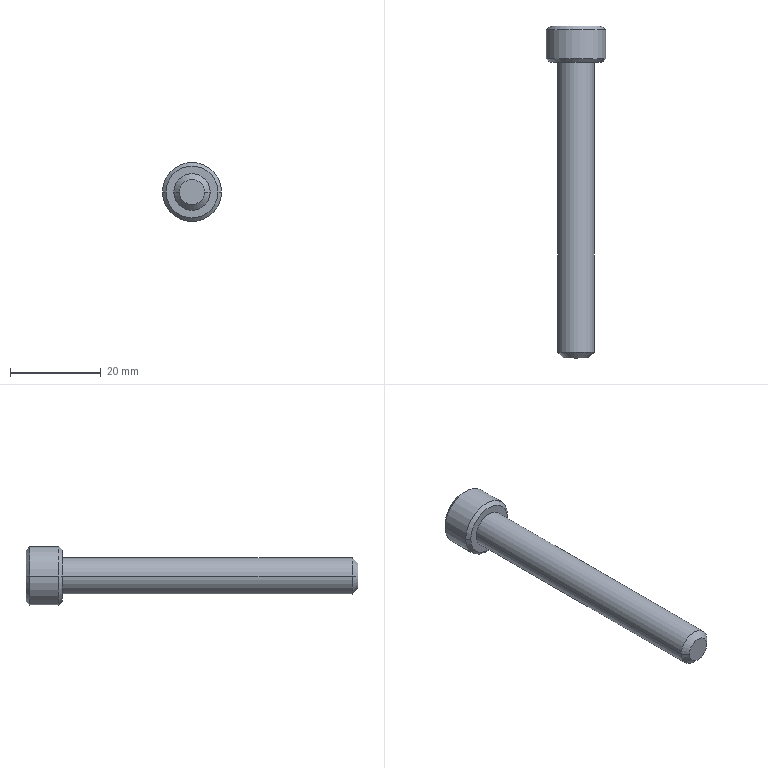Part | STEP file | BB62-M8-65L-3 | 1 solid | 27 faces | box 13 x 73 x 13 mm | volume 4140 mm3 | plane 15 | cone 8 | cylinder 4 | commonest cylinder face diameters 8 x2 13 x2
STEP:
#1=CARTESIAN_POINT('',(0.,2.02,0.));
#2=VERTEX_POINT('',#1);
#3=CARTESIAN_POINT('',(3.43,4.,0.));
#4=VERTEX_POINT('',#3);
#5=CARTESIAN_POINT('',(0.,2.02,0.));
#6=DIRECTION('',(0.866,0.5,0.));
#7=VECTOR('',#6,1000.);
#8=LINE('',#5,#7);
#9=EDGE_CURVE('',#2,#4,#8,.T.);
#10=ORIENTED_EDGE('',*,*,#9,.F.);
#11=CARTESIAN_POINT('',(-3.43,4.,0.));
#12=VERTEX_POINT('',#11);
#13=CARTESIAN_POINT('',(0.,2.02,0.));
#14=DIRECTION('',(-0.866,0.5,0.));
#15=VECTOR('',#14,1000.);
#16=LINE('',#13,#15);
#17=EDGE_CURVE('',#2,#12,#16,.T.);
#18=ORIENTED_EDGE('',*,*,#17,.T.);
#19=CARTESIAN_POINT('',(-2.97,4.,1.715));
#20=VERTEX_POINT('',#19);
#21=CARTESIAN_POINT('',(0.,4.,0.));
#22=DIRECTION('',(0.,-1.,0.));
#23=DIRECTION('',(-1.,0.,0.));
#24=AXIS2_PLACEMENT_3D('',#21,#22,#23);
#25=CIRCLE('',#24,3.43);
#26=EDGE_CURVE('',#20,#12,#25,.T.);
#27=ORIENTED_EDGE('',*,*,#26,.F.);
#28=CARTESIAN_POINT('',(0.,4.,3.43));
#29=VERTEX_POINT('',#28);
#30=CARTESIAN_POINT('',(0.,4.,0.));
#31=DIRECTION('',(0.,-1.,0.));
#32=DIRECTION('',(-1.,0.,0.));
#33=AXIS2_PLACEMENT_3D('',#30,#31,#32);
#34=CIRCLE('',#33,3.43);
#35=EDGE_CURVE('',#29,#20,#34,.T.);
#36=ORIENTED_EDGE('',*,*,#35,.F.);
#37=CARTESIAN_POINT('',(2.97,4.,1.715));
#38=VERTEX_POINT('',#37);
#39=CARTESIAN_POINT('',(0.,4.,0.));
#40=DIRECTION('',(0.,-1.,0.));
#41=DIRECTION('',(-1.,0.,0.));
#42=AXIS2_PLACEMENT_3D('',#39,#40,#41);
#43=CIRCLE('',#42,3.43);
#44=EDGE_CURVE('',#38,#29,#43,.T.);
#45=ORIENTED_EDGE('',*,*,#44,.F.);
#46=CARTESIAN_POINT('',(0.,4.,0.));
#47=DIRECTION('',(0.,-1.,0.));
#48=DIRECTION('',(-1.,0.,0.));
#49=AXIS2_PLACEMENT_3D('',#46,#47,#48);
#50=CIRCLE('',#49,3.43);
#51=EDGE_CURVE('',#4,#38,#50,.T.);
#52=ORIENTED_EDGE('',*,*,#51,.F.);
#53=EDGE_LOOP('',(#10,#18,#27,#36,#45,#52));
#54=FACE_OUTER_BOUND('',#53,.T.);
#55=CARTESIAN_POINT('',(0.,1002.02,0.));
#56=DIRECTION('',(0.,1.,0.));
#57=DIRECTION('',(1.,0.,0.));
#58=AXIS2_PLACEMENT_3D('',#55,#56,#57);
#59=CONICAL_SURFACE('',#58,1732.051,1.047);
#60=ADVANCED_FACE('',(#54),#59,.F.);
#61=CARTESIAN_POINT('',(2.75,-65.,0.));
#62=VERTEX_POINT('',#61);
#63=CARTESIAN_POINT('',(-2.75,-65.,0.));
#64=VERTEX_POINT('',#63);
#65=CARTESIAN_POINT('',(0.,-65.,0.));
#66=DIRECTION('',(0.,1.,0.));
#67=DIRECTION('',(1.,0.,0.));
#68=AXIS2_PLACEMENT_3D('',#65,#66,#67);
#69=CIRCLE('',#68,2.75);
#70=EDGE_CURVE('',#62,#64,#69,.T.);
#71=ORIENTED_EDGE('',*,*,#70,.T.);
#72=CARTESIAN_POINT('',(-4.,-63.75,0.));
#73=VERTEX_POINT('',#72);
#74=CARTESIAN_POINT('',(-2.75,-65.,0.));
#75=DIRECTION('',(-0.7071,0.7071,0.));
#76=VECTOR('',#75,1000.);
#77=LINE('',#74,#76);
#78=EDGE_CURVE('',#64,#73,#77,.T.);
#79=ORIENTED_EDGE('',*,*,#78,.T.);
#80=CARTESIAN_POINT('',(4.,-63.75,0.));
#81=VERTEX_POINT('',#80);
#82=CARTESIAN_POINT('',(0.,-63.75,0.));
#83=DIRECTION('',(0.,-1.,0.));
#84=DIRECTION('',(-1.,0.,0.));
#85=AXIS2_PLACEMENT_3D('',#82,#83,#84);
#86=CIRCLE('',#85,4.);
#87=EDGE_CURVE('',#73,#81,#86,.T.);
#88=ORIENTED_EDGE('',*,*,#87,.T.);
#89=CARTESIAN_POINT('',(2.75,-65.,0.));
#90=DIRECTION('',(0.7071,0.7071,0.));
#91=VECTOR('',#90,1000.);
#92=LINE('',#89,#91);
#93=EDGE_CURVE('',#62,#81,#92,.T.);
#94=ORIENTED_EDGE('',*,*,#93,.F.);
#95=EDGE_LOOP('',(#71,#79,#88,#94));
#96=FACE_OUTER_BOUND('',#95,.T.);
#97=CARTESIAN_POINT('',(0.,-65.,0.));
#98=DIRECTION('',(0.,1.,0.));
#99=DIRECTION('',(1.,0.,0.));
#100=AXIS2_PLACEMENT_3D('',#97,#98,#99);
#101=CONICAL_SURFACE('',#100,2.75,0.7854);
#102=ADVANCED_FACE('',(#96),#101,.T.);
#103=ORIENTED_EDGE('',*,*,#87,.F.);
#104=CARTESIAN_POINT('',(-4.,0.,0.));
#105=VERTEX_POINT('',#104);
#106=CARTESIAN_POINT('',(-4.,-63.75,0.));
#107=DIRECTION('',(0.,1.,0.));
#108=VECTOR('',#107,1000.);
#109=LINE('',#106,#108);
#110=EDGE_CURVE('',#73,#105,#109,.T.);
#111=ORIENTED_EDGE('',*,*,#110,.T.);
#112=CARTESIAN_POINT('',(4.,0.,0.));
#113=VERTEX_POINT('',#112);
#114=CARTESIAN_POINT('',(0.,0.,0.));
#115=DIRECTION('',(0.,-1.,0.));
#116=DIRECTION('',(-1.,0.,0.));
#117=AXIS2_PLACEMENT_3D('',#114,#115,#116);
#118=CIRCLE('',#117,4.);
#119=EDGE_CURVE('',#105,#113,#118,.T.);
#120=ORIENTED_EDGE('',*,*,#119,.T.);
#121=CARTESIAN_POINT('',(4.,-63.75,0.));
#122=DIRECTION('',(0.,1.,0.));
#123=VECTOR('',#122,1000.);
#124=LINE('',#121,#123);
#125=EDGE_CURVE('',#81,#113,#124,.T.);
#126=ORIENTED_EDGE('',*,*,#125,.F.);
#127=EDGE_LOOP('',(#103,#111,#120,#126));
#128=FACE_OUTER_BOUND('',#127,.T.);
#129=CARTESIAN_POINT('',(0.,-63.75,0.));
#130=DIRECTION('',(0.,1.,0.));
#131=DIRECTION('',(1.,0.,0.));
#132=AXIS2_PLACEMENT_3D('',#129,#130,#131);
#133=CYLINDRICAL_SURFACE('',#132,4.);
#134=ADVANCED_FACE('',(#128),#133,.T.);
#135=CARTESIAN_POINT('',(-5.7,8.,0.));
#136=VERTEX_POINT('',#135);
#137=CARTESIAN_POINT('',(5.7,8.,0.));
#138=VERTEX_POINT('',#137);
#139=CARTESIAN_POINT('',(0.,8.,0.));
#140=DIRECTION('',(0.,-1.,0.));
#141=DIRECTION('',(-1.,0.,0.));
#142=AXIS2_PLACEMENT_3D('',#139,#140,#141);
#143=CIRCLE('',#142,5.7);
#144=EDGE_CURVE('',#136,#138,#143,.T.);
#145=ORIENTED_EDGE('',*,*,#144,.T.);
#146=CARTESIAN_POINT('',(6.5,7.2,0.));
#147=VERTEX_POINT('',#146);
#148=CARTESIAN_POINT('',(6.5,7.2,0.));
#149=DIRECTION('',(0.7071,-0.7071,0.));
#150=VECTOR('',#149,1000.);
#151=LINE('',#148,#150);
#152=EDGE_CURVE('',#138,#147,#151,.T.);
#153=ORIENTED_EDGE('',*,*,#152,.T.);
#154=CARTESIAN_POINT('',(-6.5,7.2,0.));
#155=VERTEX_POINT('',#154);
#156=CARTESIAN_POINT('',(0.,7.2,0.));
#157=DIRECTION('',(0.,-1.,0.));
#158=DIRECTION('',(-1.,0.,0.));
#159=AXIS2_PLACEMENT_3D('',#156,#157,#158);
#160=CIRCLE('',#159,6.5);
#161=EDGE_CURVE('',#155,#147,#160,.T.);
#162=ORIENTED_EDGE('',*,*,#161,.F.);
#163=CARTESIAN_POINT('',(-6.5,7.2,0.));
#164=DIRECTION('',(-0.7071,-0.7071,0.));
#165=VECTOR('',#164,1000.);
#166=LINE('',#163,#165);
#167=EDGE_CURVE('',#136,#155,#166,.T.);
#168=ORIENTED_EDGE('',*,*,#167,.F.);
#169=EDGE_LOOP('',(#145,#153,#162,#168));
#170=FACE_OUTER_BOUND('',#169,.T.);
#171=CARTESIAN_POINT('',(0.,7.2,0.));
#172=DIRECTION('',(0.,-1.,0.));
#173=DIRECTION('',(-1.,0.,0.));
#174=AXIS2_PLACEMENT_3D('',#171,#172,#173);
#175=CONICAL_SURFACE('',#174,6.5,0.7854);
#176=ADVANCED_FACE('',(#170),#175,.T.);
#177=ORIENTED_EDGE('',*,*,#161,.T.);
#178=CARTESIAN_POINT('',(6.5,0.8,0.));
#179=VERTEX_POINT('',#178);
#180=CARTESIAN_POINT('',(6.5,1.62,0.));
#181=DIRECTION('',(0.,-1.,0.));
#182=VECTOR('',#181,1000.);
#183=LINE('',#180,#182);
#184=EDGE_CURVE('',#147,#179,#183,.T.);
#185=ORIENTED_EDGE('',*,*,#184,.T.);
#186=CARTESIAN_POINT('',(-6.5,0.8,0.));
#187=VERTEX_POINT('',#186);
#188=CARTESIAN_POINT('',(0.,0.8,0.));
#189=DIRECTION('',(0.,-1.,0.));
#190=DIRECTION('',(-1.,0.,0.));
#191=AXIS2_PLACEMENT_3D('',#188,#189,#190);
#192=CIRCLE('',#191,6.5);
#193=EDGE_CURVE('',#187,#179,#192,.T.);
#194=ORIENTED_EDGE('',*,*,#193,.F.);
#195=CARTESIAN_POINT('',(-6.5,1.62,0.));
#196=DIRECTION('',(0.,-1.,0.));
#197=VECTOR('',#196,1000.);
#198=LINE('',#195,#197);
#199=EDGE_CURVE('',#155,#187,#198,.T.);
#200=ORIENTED_EDGE('',*,*,#199,.F.);
#201=EDGE_LOOP('',(#177,#185,#194,#200));
#202=FACE_OUTER_BOUND('',#201,.T.);
#203=CARTESIAN_POINT('',(0.,1.62,0.));
#204=DIRECTION('',(0.,-1.,0.));
#205=DIRECTION('',(-1.,0.,0.));
#206=AXIS2_PLACEMENT_3D('',#203,#204,#205);
#207=CYLINDRICAL_SURFACE('',#206,6.5);
#208=ADVANCED_FACE('',(#202),#207,.T.);
#209=CARTESIAN_POINT('',(-5.7,0.,0.));
#210=VERTEX_POINT('',#209);
#211=CARTESIAN_POINT('',(5.7,0.,0.));
#212=VERTEX_POINT('',#211);
#213=CARTESIAN_POINT('',(0.,0.,0.));
#214=DIRECTION('',(0.,-1.,0.));
#215=DIRECTION('',(-1.,0.,0.));
#216=AXIS2_PLACEMENT_3D('',#213,#214,#215);
#217=CIRCLE('',#216,5.7);
#218=EDGE_CURVE('',#210,#212,#217,.T.);
#219=ORIENTED_EDGE('',*,*,#218,.F.);
#220=CARTESIAN_POINT('',(-5.7,0.,0.));
#221=DIRECTION('',(-0.7071,0.7071,0.));
#222=VECTOR('',#221,1000.);
#223=LINE('',#220,#222);
#224=EDGE_CURVE('',#210,#187,#223,.T.);
#225=ORIENTED_EDGE('',*,*,#224,.T.);
#226=ORIENTED_EDGE('',*,*,#193,.T.);
#227=CARTESIAN_POINT('',(5.7,0.,0.));
#228=DIRECTION('',(0.7071,0.7071,0.));
#229=VECTOR('',#228,1000.);
#230=LINE('',#227,#229);
#231=EDGE_CURVE('',#212,#179,#230,.T.);
#232=ORIENTED_EDGE('',*,*,#231,.F.);
#233=EDGE_LOOP('',(#219,#225,#226,#232));
#234=FACE_OUTER_BOUND('',#233,.T.);
#235=CARTESIAN_POINT('',(0.,0.,0.));
#236=DIRECTION('',(0.,1.,0.));
#237=DIRECTION('',(1.,0.,0.));
#238=AXIS2_PLACEMENT_3D('',#235,#236,#237);
#239=CONICAL_SURFACE('',#238,5.7,0.7854);
#240=ADVANCED_FACE('',(#234),#239,.T.);
#241=ORIENTED_EDGE('',*,*,#144,.F.);
#242=CARTESIAN_POINT('',(0.,8.,0.));
#243=DIRECTION('',(0.,-1.,0.));
#244=DIRECTION('',(-1.,0.,0.));
#245=AXIS2_PLACEMENT_3D('',#242,#243,#244);
#246=CIRCLE('',#245,5.7);
#247=EDGE_CURVE('',#138,#136,#246,.T.);
#248=ORIENTED_EDGE('',*,*,#247,.F.);
#249=EDGE_LOOP('',(#241,#248));
#250=FACE_OUTER_BOUND('',#249,.T.);
#251=CARTESIAN_POINT('',(0.,8.,-3.43));
#252=VERTEX_POINT('',#251);
#253=CARTESIAN_POINT('',(-2.97,8.,-1.715));
#254=VERTEX_POINT('',#253);
#255=CARTESIAN_POINT('',(0.,8.,-3.43));
#256=DIRECTION('',(-0.866,0.,0.5));
#257=VECTOR('',#256,1000.);
#258=LINE('',#255,#257);
#259=EDGE_CURVE('',#252,#254,#258,.T.);
#260=ORIENTED_EDGE('',*,*,#259,.F.);
#261=CARTESIAN_POINT('',(2.97,8.,-1.715));
#262=VERTEX_POINT('',#261);
#263=CARTESIAN_POINT('',(2.97,8.,-1.715));
#264=DIRECTION('',(-0.866,0.,-0.5));
#265=VECTOR('',#264,1000.);
#266=LINE('',#263,#265);
#267=EDGE_CURVE('',#262,#252,#266,.T.);
#268=ORIENTED_EDGE('',*,*,#267,.F.);
#269=CARTESIAN_POINT('',(2.97,8.,1.715));
#270=VERTEX_POINT('',#269);
#271=CARTESIAN_POINT('',(2.97,8.,1.715));
#272=DIRECTION('',(0.,0.,-1.));
#273=VECTOR('',#272,1000.);
#274=LINE('',#271,#273);
#275=EDGE_CURVE('',#270,#262,#274,.T.);
#276=ORIENTED_EDGE('',*,*,#275,.F.);
#277=CARTESIAN_POINT('',(0.,8.,3.43));
#278=VERTEX_POINT('',#277);
#279=CARTESIAN_POINT('',(0.,8.,3.43));
#280=DIRECTION('',(0.866,0.,-0.5));
#281=VECTOR('',#280,1000.);
#282=LINE('',#279,#281);
#283=EDGE_CURVE('',#278,#270,#282,.T.);
#284=ORIENTED_EDGE('',*,*,#283,.F.);
#285=CARTESIAN_POINT('',(-2.97,8.,1.715));
#286=VERTEX_POINT('',#285);
#287=CARTESIAN_POINT('',(-2.97,8.,1.715));
#288=DIRECTION('',(0.866,0.,0.5));
#289=VECTOR('',#288,1000.);
#290=LINE('',#287,#289);
#291=EDGE_CURVE('',#286,#278,#290,.T.);
#292=ORIENTED_EDGE('',*,*,#291,.F.);
#293=CARTESIAN_POINT('',(-2.97,8.,-1.715));
#294=DIRECTION('',(0.,0.,1.));
#295=VECTOR('',#294,1000.);
#296=LINE('',#293,#295);
#297=EDGE_CURVE('',#254,#286,#296,.T.);
#298=ORIENTED_EDGE('',*,*,#297,.F.);
#299=EDGE_LOOP('',(#260,#268,#276,#284,#292,#298));
#300=FACE_BOUND('',#299,.T.);
#301=CARTESIAN_POINT('',(5.7,8.,0.));
#302=DIRECTION('',(0.,1.,0.));
#303=DIRECTION('',(1.,0.,0.));
#304=AXIS2_PLACEMENT_3D('',#301,#302,#303);
#305=PLANE('',#304);
#306=ADVANCED_FACE('',(#250,#300),#305,.T.);
#307=CARTESIAN_POINT('',(0.,0.,0.));
#308=DIRECTION('',(0.,-1.,0.));
#309=DIRECTION('',(-1.,0.,0.));
#310=AXIS2_PLACEMENT_3D('',#307,#308,#309);
#311=CIRCLE('',#310,4.);
#312=EDGE_CURVE('',#113,#105,#311,.T.);
#313=ORIENTED_EDGE('',*,*,#312,.F.);
#314=ORIENTED_EDGE('',*,*,#119,.F.);
#315=EDGE_LOOP('',(#313,#314));
#316=FACE_BOUND('',#315,.T.);
#317=CARTESIAN_POINT('',(0.,0.,0.));
#318=DIRECTION('',(0.,-1.,0.));
#319=DIRECTION('',(-1.,0.,0.));
#320=AXIS2_PLACEMENT_3D('',#317,#318,#319);
#321=CIRCLE('',#320,5.7);
#322=EDGE_CURVE('',#212,#210,#321,.T.);
#323=ORIENTED_EDGE('',*,*,#322,.T.);
#324=ORIENTED_EDGE('',*,*,#218,.T.);
#325=EDGE_LOOP('',(#323,#324));
#326=FACE_OUTER_BOUND('',#325,.T.);
#327=CARTESIAN_POINT('',(0.,0.,0.));
#328=DIRECTION('',(0.,-1.,0.));
#329=DIRECTION('',(-1.,0.,0.));
#330=AXIS2_PLACEMENT_3D('',#327,#328,#329);
#331=PLANE('',#330);
#332=ADVANCED_FACE('',(#316,#326),#331,.T.);
#333=ORIENTED_EDGE('',*,*,#224,.F.);
#334=ORIENTED_EDGE('',*,*,#322,.F.);
#335=ORIENTED_EDGE('',*,*,#231,.T.);
#336=CARTESIAN_POINT('',(0.,0.8,0.));
#337=DIRECTION('',(0.,-1.,0.));
#338=DIRECTION('',(-1.,0.,0.));
#339=AXIS2_PLACEMENT_3D('',#336,#337,#338);
#340=CIRCLE('',#339,6.5);
#341=EDGE_CURVE('',#179,#187,#340,.T.);
#342=ORIENTED_EDGE('',*,*,#341,.T.);
#343=EDGE_LOOP('',(#333,#334,#335,#342));
#344=FACE_OUTER_BOUND('',#343,.T.);
#345=CARTESIAN_POINT('',(0.,0.,0.));
#346=DIRECTION('',(0.,1.,0.));
#347=DIRECTION('',(1.,0.,0.));
#348=AXIS2_PLACEMENT_3D('',#345,#346,#347);
#349=CONICAL_SURFACE('',#348,5.7,0.7854);
#350=ADVANCED_FACE('',(#344),#349,.T.);
#351=ORIENTED_EDGE('',*,*,#184,.F.);
#352=CARTESIAN_POINT('',(0.,7.2,0.));
#353=DIRECTION('',(0.,-1.,0.));
#354=DIRECTION('',(-1.,0.,0.));
#355=AXIS2_PLACEMENT_3D('',#352,#353,#354);
#356=CIRCLE('',#355,6.5);
#357=EDGE_CURVE('',#147,#155,#356,.T.);
#358=ORIENTED_EDGE('',*,*,#357,.T.);
#359=ORIENTED_EDGE('',*,*,#199,.T.);
#360=ORIENTED_EDGE('',*,*,#341,.F.);
#361=EDGE_LOOP('',(#351,#358,#359,#360));
#362=FACE_OUTER_BOUND('',#361,.T.);
#363=CARTESIAN_POINT('',(0.,1.62,0.));
#364=DIRECTION('',(0.,-1.,0.));
#365=DIRECTION('',(-1.,0.,0.));
#366=AXIS2_PLACEMENT_3D('',#363,#364,#365);
#367=CYLINDRICAL_SURFACE('',#366,6.5);
#368=ADVANCED_FACE('',(#362),#367,.T.);
#369=ORIENTED_EDGE('',*,*,#152,.F.);
#370=ORIENTED_EDGE('',*,*,#247,.T.);
#371=ORIENTED_EDGE('',*,*,#167,.T.);
#372=ORIENTED_EDGE('',*,*,#357,.F.);
#373=EDGE_LOOP('',(#369,#370,#371,#372));
#374=FACE_OUTER_BOUND('',#373,.T.);
#375=CARTESIAN_POINT('',(0.,7.2,0.));
#376=DIRECTION('',(0.,-1.,0.));
#377=DIRECTION('',(-1.,0.,0.));
#378=AXIS2_PLACEMENT_3D('',#375,#376,#377);
#379=CONICAL_SURFACE('',#378,6.5,0.7854);
#380=ADVANCED_FACE('',(#374),#379,.T.);
#381=ORIENTED_EDGE('',*,*,#110,.F.);
#382=CARTESIAN_POINT('',(0.,-63.75,0.));
#383=DIRECTION('',(0.,-1.,0.));
#384=DIRECTION('',(-1.,0.,0.));
#385=AXIS2_PLACEMENT_3D('',#382,#383,#384);
#386=CIRCLE('',#385,4.);
#387=EDGE_CURVE('',#81,#73,#386,.T.);
#388=ORIENTED_EDGE('',*,*,#387,.F.);
#389=ORIENTED_EDGE('',*,*,#125,.T.);
#390=ORIENTED_EDGE('',*,*,#312,.T.);
#391=EDGE_LOOP('',(#381,#388,#389,#390));
#392=FACE_OUTER_BOUND('',#391,.T.);
#393=CARTESIAN_POINT('',(0.,-63.75,0.));
#394=DIRECTION('',(0.,1.,0.));
#395=DIRECTION('',(1.,0.,0.));
#396=AXIS2_PLACEMENT_3D('',#393,#394,#395);
#397=CYLINDRICAL_SURFACE('',#396,4.);
#398=ADVANCED_FACE('',(#392),#397,.T.);
#399=ORIENTED_EDGE('',*,*,#70,.F.);
#400=CARTESIAN_POINT('',(0.,-65.,0.));
#401=DIRECTION('',(0.,1.,0.));
#402=DIRECTION('',(1.,0.,0.));
#403=AXIS2_PLACEMENT_3D('',#400,#401,#402);
#404=CIRCLE('',#403,2.75);
#405=EDGE_CURVE('',#64,#62,#404,.T.);
#406=ORIENTED_EDGE('',*,*,#405,.F.);
#407=EDGE_LOOP('',(#399,#406));
#408=FACE_OUTER_BOUND('',#407,.T.);
#409=CARTESIAN_POINT('',(0.,-65.,0.));
#410=DIRECTION('',(0.,-1.,0.));
#411=DIRECTION('',(-1.,0.,0.));
#412=AXIS2_PLACEMENT_3D('',#409,#410,#411);
#413=PLANE('',#412);
#414=ADVANCED_FACE('',(#408),#413,.T.);
#415=ORIENTED_EDGE('',*,*,#78,.F.);
#416=ORIENTED_EDGE('',*,*,#405,.T.);
#417=ORIENTED_EDGE('',*,*,#93,.T.);
#418=ORIENTED_EDGE('',*,*,#387,.T.);
#419=EDGE_LOOP('',(#415,#416,#417,#418));
#420=FACE_OUTER_BOUND('',#419,.T.);
#421=CARTESIAN_POINT('',(0.,-65.,0.));
#422=DIRECTION('',(0.,1.,0.));
#423=DIRECTION('',(1.,0.,0.));
#424=AXIS2_PLACEMENT_3D('',#421,#422,#423);
#425=CONICAL_SURFACE('',#424,2.75,0.7854);
#426=ADVANCED_FACE('',(#420),#425,.T.);
#427=CARTESIAN_POINT('',(2.97,4.,-1.715));
#428=VERTEX_POINT('',#427);
#429=CARTESIAN_POINT('',(0.,4.,-3.43));
#430=VERTEX_POINT('',#429);
#431=CARTESIAN_POINT('',(2.97,4.,-1.715));
#432=DIRECTION('',(-0.866,0.,-0.5));
#433=VECTOR('',#432,1000.);
#434=LINE('',#431,#433);
#435=EDGE_CURVE('',#428,#430,#434,.T.);
#436=ORIENTED_EDGE('',*,*,#435,.F.);
#437=CARTESIAN_POINT('',(2.97,8.,-1.715));
#438=DIRECTION('',(0.,-1.,0.));
#439=VECTOR('',#438,1000.);
#440=LINE('',#437,#439);
#441=EDGE_CURVE('',#262,#428,#440,.T.);
#442=ORIENTED_EDGE('',*,*,#441,.F.);
#443=ORIENTED_EDGE('',*,*,#267,.T.);
#444=CARTESIAN_POINT('',(0.,8.,-3.43));
#445=DIRECTION('',(0.,-1.,0.));
#446=VECTOR('',#445,1000.);
#447=LINE('',#444,#446);
#448=EDGE_CURVE('',#252,#430,#447,.T.);
#449=ORIENTED_EDGE('',*,*,#448,.T.);
#450=EDGE_LOOP('',(#436,#442,#443,#449));
#451=FACE_OUTER_BOUND('',#450,.T.);
#452=CARTESIAN_POINT('',(2.97,8.,-1.715));
#453=DIRECTION('',(-0.5,0.,0.866));
#454=DIRECTION('',(0.866,0.,0.5));
#455=AXIS2_PLACEMENT_3D('',#452,#453,#454);
#456=PLANE('',#455);
#457=ADVANCED_FACE('',(#451),#456,.T.);
#458=CARTESIAN_POINT('',(-2.97,4.,-1.715));
#459=VERTEX_POINT('',#458);
#460=CARTESIAN_POINT('',(0.,4.,-3.43));
#461=DIRECTION('',(-0.866,0.,0.5));
#462=VECTOR('',#461,1000.);
#463=LINE('',#460,#462);
#464=EDGE_CURVE('',#430,#459,#463,.T.);
#465=ORIENTED_EDGE('',*,*,#464,.F.);
#466=ORIENTED_EDGE('',*,*,#448,.F.);
#467=ORIENTED_EDGE('',*,*,#259,.T.);
#468=CARTESIAN_POINT('',(-2.97,8.,-1.715));
#469=DIRECTION('',(0.,-1.,0.));
#470=VECTOR('',#469,1000.);
#471=LINE('',#468,#470);
#472=EDGE_CURVE('',#254,#459,#471,.T.);
#473=ORIENTED_EDGE('',*,*,#472,.T.);
#474=EDGE_LOOP('',(#465,#466,#467,#473));
#475=FACE_OUTER_BOUND('',#474,.T.);
#476=CARTESIAN_POINT('',(0.,8.,-3.43));
#477=DIRECTION('',(0.5,0.,0.866));
#478=DIRECTION('',(0.866,0.,-0.5));
#479=AXIS2_PLACEMENT_3D('',#476,#477,#478);
#480=PLANE('',#479);
#481=ADVANCED_FACE('',(#475),#480,.T.);
#482=CARTESIAN_POINT('',(-2.97,4.,-1.715));
#483=DIRECTION('',(0.,0.,1.));
#484=VECTOR('',#483,1000.);
#485=LINE('',#482,#484);
#486=EDGE_CURVE('',#459,#20,#485,.T.);
#487=ORIENTED_EDGE('',*,*,#486,.F.);
#488=ORIENTED_EDGE('',*,*,#472,.F.);
#489=ORIENTED_EDGE('',*,*,#297,.T.);
#490=CARTESIAN_POINT('',(-2.97,8.,1.715));
#491=DIRECTION('',(0.,-1.,0.));
#492=VECTOR('',#491,1000.);
#493=LINE('',#490,#492);
#494=EDGE_CURVE('',#286,#20,#493,.T.);
#495=ORIENTED_EDGE('',*,*,#494,.T.);
#496=EDGE_LOOP('',(#487,#488,#489,#495));
#497=FACE_OUTER_BOUND('',#496,.T.);
#498=CARTESIAN_POINT('',(-2.97,8.,-1.715));
#499=DIRECTION('',(1.,0.,0.));
#500=DIRECTION('',(0.,0.,-1.));
#501=AXIS2_PLACEMENT_3D('',#498,#499,#500);
#502=PLANE('',#501);
#503=ADVANCED_FACE('',(#497),#502,.T.);
#504=CARTESIAN_POINT('',(-2.97,4.,1.715));
#505=DIRECTION('',(0.866,0.,0.5));
#506=VECTOR('',#505,1000.);
#507=LINE('',#504,#506);
#508=EDGE_CURVE('',#20,#29,#507,.T.);
#509=ORIENTED_EDGE('',*,*,#508,.F.);
#510=ORIENTED_EDGE('',*,*,#494,.F.);
#511=ORIENTED_EDGE('',*,*,#291,.T.);
#512=CARTESIAN_POINT('',(0.,8.,3.43));
#513=DIRECTION('',(0.,-1.,0.));
#514=VECTOR('',#513,1000.);
#515=LINE('',#512,#514);
#516=EDGE_CURVE('',#278,#29,#515,.T.);
#517=ORIENTED_EDGE('',*,*,#516,.T.);
#518=EDGE_LOOP('',(#509,#510,#511,#517));
#519=FACE_OUTER_BOUND('',#518,.T.);
#520=CARTESIAN_POINT('',(-2.97,8.,1.715));
#521=DIRECTION('',(0.5,0.,-0.866));
#522=DIRECTION('',(-0.866,0.,-0.5));
#523=AXIS2_PLACEMENT_3D('',#520,#521,#522);
#524=PLANE('',#523);
#525=ADVANCED_FACE('',(#519),#524,.T.);
#526=CARTESIAN_POINT('',(0.,4.,3.43));
#527=DIRECTION('',(0.866,0.,-0.5));
#528=VECTOR('',#527,1000.);
#529=LINE('',#526,#528);
#530=EDGE_CURVE('',#29,#38,#529,.T.);
#531=ORIENTED_EDGE('',*,*,#530,.F.);
#532=ORIENTED_EDGE('',*,*,#516,.F.);
#533=ORIENTED_EDGE('',*,*,#283,.T.);
#534=CARTESIAN_POINT('',(2.97,8.,1.715));
#535=DIRECTION('',(0.,-1.,0.));
#536=VECTOR('',#535,1000.);
#537=LINE('',#534,#536);
#538=EDGE_CURVE('',#270,#38,#537,.T.);
#539=ORIENTED_EDGE('',*,*,#538,.T.);
#540=EDGE_LOOP('',(#531,#532,#533,#539));
#541=FACE_OUTER_BOUND('',#540,.T.);
#542=CARTESIAN_POINT('',(0.,8.,3.43));
#543=DIRECTION('',(-0.5,0.,-0.866));
#544=DIRECTION('',(-0.866,0.,0.5));
#545=AXIS2_PLACEMENT_3D('',#542,#543,#544);
#546=PLANE('',#545);
#547=ADVANCED_FACE('',(#541),#546,.T.);
#548=CARTESIAN_POINT('',(2.97,4.,1.715));
#549=DIRECTION('',(0.,0.,-1.));
#550=VECTOR('',#549,1000.);
#551=LINE('',#548,#550);
#552=EDGE_CURVE('',#38,#428,#551,.T.);
#553=ORIENTED_EDGE('',*,*,#552,.F.);
#554=ORIENTED_EDGE('',*,*,#538,.F.);
#555=ORIENTED_EDGE('',*,*,#275,.T.);
#556=ORIENTED_EDGE('',*,*,#441,.T.);
#557=EDGE_LOOP('',(#553,#554,#555,#556));
#558=FACE_OUTER_BOUND('',#557,.T.);
#559=CARTESIAN_POINT('',(2.97,8.,1.715));
#560=DIRECTION('',(-1.,0.,0.));
#561=DIRECTION('',(0.,0.,1.));
#562=AXIS2_PLACEMENT_3D('',#559,#560,#561);
#563=PLANE('',#562);
#564=ADVANCED_FACE('',(#558),#563,.T.);
#565=ORIENTED_EDGE('',*,*,#435,.T.);
#566=CARTESIAN_POINT('',(0.,4.,0.));
#567=DIRECTION('',(0.,-1.,0.));
#568=DIRECTION('',(-1.,0.,0.));
#569=AXIS2_PLACEMENT_3D('',#566,#567,#568);
#570=CIRCLE('',#569,3.43);
#571=EDGE_CURVE('',#430,#428,#570,.T.);
#572=ORIENTED_EDGE('',*,*,#571,.T.);
#573=EDGE_LOOP('',(#565,#572));
#574=FACE_OUTER_BOUND('',#573,.T.);
#575=CARTESIAN_POINT('',(0.,4.,0.));
#576=DIRECTION('',(0.,1.,0.));
#577=DIRECTION('',(1.,0.,0.));
#578=AXIS2_PLACEMENT_3D('',#575,#576,#577);
#579=PLANE('',#578);
#580=ADVANCED_FACE('',(#574),#579,.F.);
#581=ORIENTED_EDGE('',*,*,#552,.T.);
#582=CARTESIAN_POINT('',(0.,4.,0.));
#583=DIRECTION('',(0.,-1.,0.));
#584=DIRECTION('',(-1.,0.,0.));
#585=AXIS2_PLACEMENT_3D('',#582,#583,#584);
#586=CIRCLE('',#585,3.43);
#587=EDGE_CURVE('',#428,#4,#586,.T.);
#588=ORIENTED_EDGE('',*,*,#587,.T.);
#589=ORIENTED_EDGE('',*,*,#51,.T.);
#590=EDGE_LOOP('',(#581,#588,#589));
#591=FACE_OUTER_BOUND('',#590,.T.);
#592=CARTESIAN_POINT('',(0.,4.,0.));
#593=DIRECTION('',(0.,1.,0.));
#594=DIRECTION('',(1.,0.,0.));
#595=AXIS2_PLACEMENT_3D('',#592,#593,#594);
#596=PLANE('',#595);
#597=ADVANCED_FACE('',(#591),#596,.F.);
#598=ORIENTED_EDGE('',*,*,#530,.T.);
#599=ORIENTED_EDGE('',*,*,#44,.T.);
#600=EDGE_LOOP('',(#598,#599));
#601=FACE_OUTER_BOUND('',#600,.T.);
#602=CARTESIAN_POINT('',(0.,4.,0.));
#603=DIRECTION('',(0.,1.,0.));
#604=DIRECTION('',(1.,0.,0.));
#605=AXIS2_PLACEMENT_3D('',#602,#603,#604);
#606=PLANE('',#605);
#607=ADVANCED_FACE('',(#601),#606,.F.);
#608=ORIENTED_EDGE('',*,*,#508,.T.);
#609=ORIENTED_EDGE('',*,*,#35,.T.);
#610=EDGE_LOOP('',(#608,#609));
#611=FACE_OUTER_BOUND('',#610,.T.);
#612=CARTESIAN_POINT('',(0.,4.,0.));
#613=DIRECTION('',(0.,1.,0.));
#614=DIRECTION('',(1.,0.,0.));
#615=AXIS2_PLACEMENT_3D('',#612,#613,#614);
#616=PLANE('',#615);
#617=ADVANCED_FACE('',(#611),#616,.F.);
#618=ORIENTED_EDGE('',*,*,#486,.T.);
#619=ORIENTED_EDGE('',*,*,#26,.T.);
#620=CARTESIAN_POINT('',(0.,4.,0.));
#621=DIRECTION('',(0.,-1.,0.));
#622=DIRECTION('',(-1.,0.,0.));
#623=AXIS2_PLACEMENT_3D('',#620,#621,#622);
#624=CIRCLE('',#623,3.43);
#625=EDGE_CURVE('',#12,#459,#624,.T.);
#626=ORIENTED_EDGE('',*,*,#625,.T.);
#627=EDGE_LOOP('',(#618,#619,#626));
#628=FACE_OUTER_BOUND('',#627,.T.);
#629=CARTESIAN_POINT('',(0.,4.,0.));
#630=DIRECTION('',(0.,1.,0.));
#631=DIRECTION('',(1.,0.,0.));
#632=AXIS2_PLACEMENT_3D('',#629,#630,#631);
#633=PLANE('',#632);
#634=ADVANCED_FACE('',(#628),#633,.F.);
#635=ORIENTED_EDGE('',*,*,#464,.T.);
#636=CARTESIAN_POINT('',(0.,4.,0.));
#637=DIRECTION('',(0.,-1.,0.));
#638=DIRECTION('',(-1.,0.,0.));
#639=AXIS2_PLACEMENT_3D('',#636,#637,#638);
#640=CIRCLE('',#639,3.43);
#641=EDGE_CURVE('',#459,#430,#640,.T.);
#642=ORIENTED_EDGE('',*,*,#641,.T.);
#643=EDGE_LOOP('',(#635,#642));
#644=FACE_OUTER_BOUND('',#643,.T.);
#645=CARTESIAN_POINT('',(0.,4.,0.));
#646=DIRECTION('',(0.,1.,0.));
#647=DIRECTION('',(1.,0.,0.));
#648=AXIS2_PLACEMENT_3D('',#645,#646,#647);
#649=PLANE('',#648);
#650=ADVANCED_FACE('',(#644),#649,.F.);
#651=ORIENTED_EDGE('',*,*,#17,.F.);
#652=ORIENTED_EDGE('',*,*,#9,.T.);
#653=ORIENTED_EDGE('',*,*,#587,.F.);
#654=ORIENTED_EDGE('',*,*,#571,.F.);
#655=ORIENTED_EDGE('',*,*,#641,.F.);
#656=ORIENTED_EDGE('',*,*,#625,.F.);
#657=EDGE_LOOP('',(#651,#652,#653,#654,#655,#656));
#658=FACE_OUTER_BOUND('',#657,.T.);
#659=CARTESIAN_POINT('',(0.,1002.02,0.));
#660=DIRECTION('',(0.,1.,0.));
#661=DIRECTION('',(1.,0.,0.));
#662=AXIS2_PLACEMENT_3D('',#659,#660,#661);
#663=CONICAL_SURFACE('',#662,1732.051,1.047);
#664=ADVANCED_FACE('',(#658),#663,.F.);
#665=CLOSED_SHELL('',(#60,#102,#134,#176,#208,#240,#306,#332,#350,#368,#380,#398,#414,#426,#457,#481,#503,#525,#547,#564,#580,#597,#607,#617,#634,#650,#664));
#666=MANIFOLD_SOLID_BREP('',#665);
#667=CARTESIAN_POINT('',(0.,0.,0.));
#668=DIRECTION('',(0.,0.,1.));
#669=DIRECTION('',(1.,0.,0.));
#670=AXIS2_PLACEMENT_3D('',#667,#668,#669);
#671=(LENGTH_UNIT()NAMED_UNIT(*)SI_UNIT(.MILLI.,.METRE.));
#672=UNCERTAINTY_MEASURE_WITH_UNIT(LENGTH_MEASURE(0.00001),#671,'','');
#673=(NAMED_UNIT(*)PLANE_ANGLE_UNIT()SI_UNIT($,.RADIAN.));
#674=(NAMED_UNIT(*)SI_UNIT($,.STERADIAN.)SOLID_ANGLE_UNIT());
#675=(GEOMETRIC_REPRESENTATION_CONTEXT(3)GLOBAL_UNCERTAINTY_ASSIGNED_CONTEXT((#672))GLOBAL_UNIT_ASSIGNED_CONTEXT((#671,#673,#674))REPRESENTATION_CONTEXT('',''));
#676=ADVANCED_BREP_SHAPE_REPRESENTATION('',(#666,#670),#675);